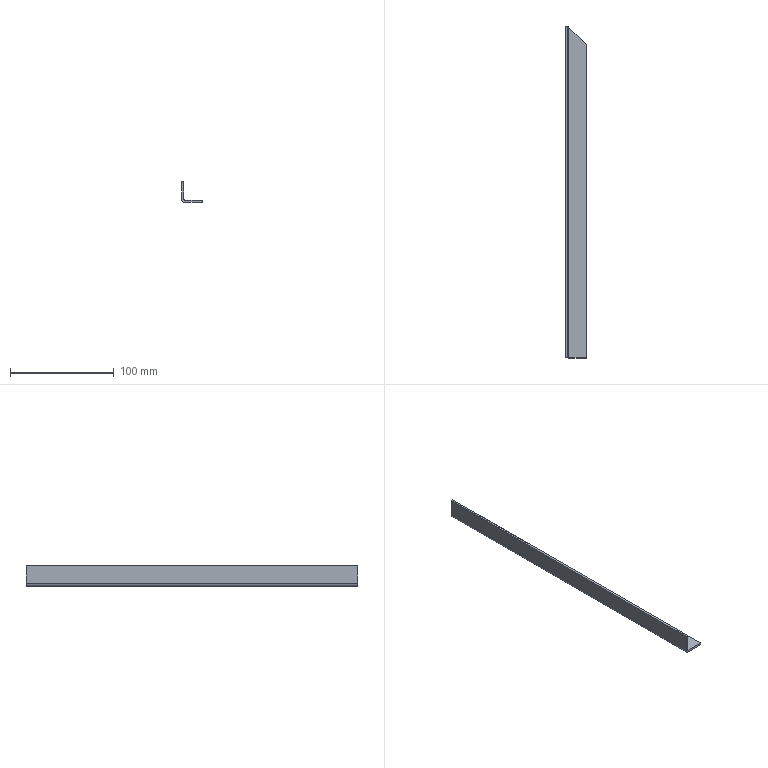Part | STEP file | Rear Closing Plate Frame Lower 3 | 1 solid | 12 faces | box 20 x 320 x 20 mm | volume 23444 mm3 | plane 9 | cylinder 2 | spline 1 | commonest cylinder face diameters 2 x1 6 x1
STEP:
#1=CARTESIAN_POINT('',(-1.251,25.392,3.));
#2=VERTEX_POINT('',#1);
#3=CARTESIAN_POINT('',(-1.251,25.392,20.));
#4=VERTEX_POINT('',#3);
#5=CARTESIAN_POINT('',(-1.251,25.392,0.));
#6=DIRECTION('',(0.,0.,1.));
#7=VECTOR('',#6,1000.);
#8=LINE('',#5,#7);
#9=EDGE_CURVE('',#2,#4,#8,.T.);
#10=ORIENTED_EDGE('',*,*,#9,.T.);
#11=CARTESIAN_POINT('',(-1.251,-294.608,20.));
#12=VERTEX_POINT('',#11);
#13=CARTESIAN_POINT('',(-1.251,0.,20.));
#14=DIRECTION('',(0.,-1.,0.));
#15=VECTOR('',#14,1000.);
#16=LINE('',#13,#15);
#17=EDGE_CURVE('',#4,#12,#16,.T.);
#18=ORIENTED_EDGE('',*,*,#17,.T.);
#19=CARTESIAN_POINT('',(-1.251,-294.608,3.));
#20=VERTEX_POINT('',#19);
#21=CARTESIAN_POINT('',(-1.251,-294.608,0.));
#22=DIRECTION('',(0.,0.,-1.));
#23=VECTOR('',#22,1000.);
#24=LINE('',#21,#23);
#25=EDGE_CURVE('',#12,#20,#24,.T.);
#26=ORIENTED_EDGE('',*,*,#25,.T.);
#27=CARTESIAN_POINT('',(-1.251,0.,3.));
#28=DIRECTION('',(0.,1.,0.));
#29=VECTOR('',#28,1000.);
#30=LINE('',#27,#29);
#31=EDGE_CURVE('',#20,#2,#30,.T.);
#32=ORIENTED_EDGE('',*,*,#31,.T.);
#33=EDGE_LOOP('',(#10,#18,#26,#32));
#34=FACE_OUTER_BOUND('',#33,.T.);
#35=CARTESIAN_POINT('',(-1.251,0.,0.));
#36=DIRECTION('',(1.,0.,0.));
#37=DIRECTION('',(0.,0.,-1.));
#38=AXIS2_PLACEMENT_3D('',#35,#36,#37);
#39=PLANE('',#38);
#40=ADVANCED_FACE('',(#34),#39,.T.);
#41=CARTESIAN_POINT('',(-3.251,25.392,20.));
#42=VERTEX_POINT('',#41);
#43=CARTESIAN_POINT('',(-3.251,25.392,20.));
#44=DIRECTION('',(1.,0.,0.));
#45=VECTOR('',#44,1000.);
#46=LINE('',#43,#45);
#47=EDGE_CURVE('',#42,#4,#46,.T.);
#48=ORIENTED_EDGE('',*,*,#47,.F.);
#49=CARTESIAN_POINT('',(-3.251,-294.608,20.));
#50=VERTEX_POINT('',#49);
#51=CARTESIAN_POINT('',(-3.251,25.392,20.));
#52=DIRECTION('',(0.,1.,0.));
#53=VECTOR('',#52,1000.);
#54=LINE('',#51,#53);
#55=EDGE_CURVE('',#50,#42,#54,.T.);
#56=ORIENTED_EDGE('',*,*,#55,.F.);
#57=CARTESIAN_POINT('',(-3.251,-294.608,20.));
#58=DIRECTION('',(-1.,0.,0.));
#59=VECTOR('',#58,1000.);
#60=LINE('',#57,#59);
#61=EDGE_CURVE('',#12,#50,#60,.T.);
#62=ORIENTED_EDGE('',*,*,#61,.F.);
#63=ORIENTED_EDGE('',*,*,#17,.F.);
#64=EDGE_LOOP('',(#48,#56,#62,#63));
#65=FACE_OUTER_BOUND('',#64,.T.);
#66=CARTESIAN_POINT('',(-3.251,25.392,20.));
#67=DIRECTION('',(0.,0.,-1.));
#68=DIRECTION('',(-1.,0.,0.));
#69=AXIS2_PLACEMENT_3D('',#66,#67,#68);
#70=PLANE('',#69);
#71=ADVANCED_FACE('',(#65),#70,.F.);
#72=CARTESIAN_POINT('',(-3.251,25.392,3.));
#73=VERTEX_POINT('',#72);
#74=CARTESIAN_POINT('',(-3.251,25.392,2.));
#75=DIRECTION('',(0.,0.,-1.));
#76=VECTOR('',#75,1000.);
#77=LINE('',#74,#76);
#78=EDGE_CURVE('',#42,#73,#77,.T.);
#79=ORIENTED_EDGE('',*,*,#78,.F.);
#80=ORIENTED_EDGE('',*,*,#47,.T.);
#81=ORIENTED_EDGE('',*,*,#9,.F.);
#82=CARTESIAN_POINT('',(-3.251,25.392,3.));
#83=DIRECTION('',(1.,0.,0.));
#84=VECTOR('',#83,1000.);
#85=LINE('',#82,#84);
#86=EDGE_CURVE('',#73,#2,#85,.T.);
#87=ORIENTED_EDGE('',*,*,#86,.F.);
#88=EDGE_LOOP('',(#79,#80,#81,#87));
#89=FACE_OUTER_BOUND('',#88,.T.);
#90=CARTESIAN_POINT('',(-3.251,25.392,2.));
#91=DIRECTION('',(0.,-1.,0.));
#92=DIRECTION('',(1.,0.,0.));
#93=AXIS2_PLACEMENT_3D('',#90,#91,#92);
#94=PLANE('',#93);
#95=ADVANCED_FACE('',(#89),#94,.F.);
#96=CARTESIAN_POINT('',(-0.2512,24.392,2.));
#97=VERTEX_POINT('',#96);
#98=CARTESIAN_POINT('',(-1.251,25.392,3.));
#99=CARTESIAN_POINT('',(-1.251,25.308,2.868));
#100=CARTESIAN_POINT('',(-1.226,25.226,2.74));
#101=CARTESIAN_POINT('',(-1.125,25.059,2.497));
#102=CARTESIAN_POINT('',(-1.052,24.976,2.387));
#103=CARTESIAN_POINT('',(-0.7735,24.725,2.108));
#104=CARTESIAN_POINT('',(-0.5154,24.56,2.));
#105=CARTESIAN_POINT('',(-0.2512,24.392,2.));
#106=B_SPLINE_CURVE_WITH_KNOTS('',3,(#98,#99,#100,#101,#102,#103,#104,#105),.UNSPECIFIED.,.F.,.F.,(4,2,2,4),(0.,0.0004622,0.0009244,0.001849),.UNSPECIFIED.);
#107=EDGE_CURVE('',#2,#97,#106,.T.);
#108=ORIENTED_EDGE('',*,*,#107,.F.);
#109=ORIENTED_EDGE('',*,*,#31,.F.);
#110=CARTESIAN_POINT('',(-0.2512,-294.608,2.));
#111=VERTEX_POINT('',#110);
#112=CARTESIAN_POINT('',(-0.2512,-294.608,3.));
#113=DIRECTION('',(0.,-1.,0.));
#114=DIRECTION('',(1.,0.,0.));
#115=AXIS2_PLACEMENT_3D('',#112,#113,#114);
#116=CIRCLE('',#115,1.);
#117=EDGE_CURVE('',#20,#111,#116,.T.);
#118=ORIENTED_EDGE('',*,*,#117,.T.);
#119=CARTESIAN_POINT('',(-0.2512,-294.608,2.));
#120=DIRECTION('',(0.,-1.,0.));
#121=VECTOR('',#120,1000.);
#122=LINE('',#119,#121);
#123=EDGE_CURVE('',#97,#111,#122,.T.);
#124=ORIENTED_EDGE('',*,*,#123,.F.);
#125=EDGE_LOOP('',(#108,#109,#118,#124));
#126=FACE_OUTER_BOUND('',#125,.T.);
#127=CARTESIAN_POINT('',(-0.2512,-294.608,3.));
#128=DIRECTION('',(0.,-1.,0.));
#129=DIRECTION('',(1.,0.,0.));
#130=AXIS2_PLACEMENT_3D('',#127,#128,#129);
#131=CYLINDRICAL_SURFACE('',#130,1.);
#132=ADVANCED_FACE('',(#126),#131,.F.);
#133=ORIENTED_EDGE('',*,*,#25,.F.);
#134=ORIENTED_EDGE('',*,*,#61,.T.);
#135=CARTESIAN_POINT('',(-3.251,-294.608,3.));
#136=VERTEX_POINT('',#135);
#137=CARTESIAN_POINT('',(-3.251,-294.608,20.));
#138=DIRECTION('',(0.,0.,1.));
#139=VECTOR('',#138,1000.);
#140=LINE('',#137,#139);
#141=EDGE_CURVE('',#136,#50,#140,.T.);
#142=ORIENTED_EDGE('',*,*,#141,.F.);
#143=CARTESIAN_POINT('',(-0.2512,-294.608,0.));
#144=VERTEX_POINT('',#143);
#145=CARTESIAN_POINT('',(-0.2512,-294.608,3.));
#146=DIRECTION('',(0.,1.,0.));
#147=DIRECTION('',(1.,0.,0.));
#148=AXIS2_PLACEMENT_3D('',#145,#146,#147);
#149=CIRCLE('',#148,3.);
#150=EDGE_CURVE('',#144,#136,#149,.T.);
#151=ORIENTED_EDGE('',*,*,#150,.F.);
#152=CARTESIAN_POINT('',(16.749,-294.608,0.));
#153=VERTEX_POINT('',#152);
#154=CARTESIAN_POINT('',(-3.251,-294.608,0.));
#155=DIRECTION('',(-1.,0.,0.));
#156=VECTOR('',#155,1000.);
#157=LINE('',#154,#156);
#158=EDGE_CURVE('',#153,#144,#157,.T.);
#159=ORIENTED_EDGE('',*,*,#158,.F.);
#160=CARTESIAN_POINT('',(16.749,-294.608,2.));
#161=VERTEX_POINT('',#160);
#162=CARTESIAN_POINT('',(16.749,-294.608,0.));
#163=DIRECTION('',(0.,0.,-1.));
#164=VECTOR('',#163,1000.);
#165=LINE('',#162,#164);
#166=EDGE_CURVE('',#161,#153,#165,.T.);
#167=ORIENTED_EDGE('',*,*,#166,.F.);
#168=CARTESIAN_POINT('',(0.,-294.608,2.));
#169=DIRECTION('',(-1.,0.,0.));
#170=VECTOR('',#169,1000.);
#171=LINE('',#168,#170);
#172=EDGE_CURVE('',#161,#111,#171,.T.);
#173=ORIENTED_EDGE('',*,*,#172,.T.);
#174=ORIENTED_EDGE('',*,*,#117,.F.);
#175=EDGE_LOOP('',(#133,#134,#142,#151,#159,#167,#173,#174));
#176=FACE_OUTER_BOUND('',#175,.T.);
#177=CARTESIAN_POINT('',(-3.251,-294.608,20.));
#178=DIRECTION('',(0.,1.,0.));
#179=DIRECTION('',(-1.,0.,0.));
#180=AXIS2_PLACEMENT_3D('',#177,#178,#179);
#181=PLANE('',#180);
#182=ADVANCED_FACE('',(#176),#181,.F.);
#183=ORIENTED_EDGE('',*,*,#141,.T.);
#184=ORIENTED_EDGE('',*,*,#55,.T.);
#185=ORIENTED_EDGE('',*,*,#78,.T.);
#186=CARTESIAN_POINT('',(-3.251,0.,3.));
#187=DIRECTION('',(0.,1.,0.));
#188=VECTOR('',#187,1000.);
#189=LINE('',#186,#188);
#190=EDGE_CURVE('',#136,#73,#189,.T.);
#191=ORIENTED_EDGE('',*,*,#190,.F.);
#192=EDGE_LOOP('',(#183,#184,#185,#191));
#193=FACE_OUTER_BOUND('',#192,.T.);
#194=CARTESIAN_POINT('',(-3.251,0.,0.));
#195=DIRECTION('',(1.,0.,0.));
#196=DIRECTION('',(0.,0.,-1.));
#197=AXIS2_PLACEMENT_3D('',#194,#195,#196);
#198=PLANE('',#197);
#199=ADVANCED_FACE('',(#193),#198,.F.);
#200=ORIENTED_EDGE('',*,*,#107,.T.);
#201=CARTESIAN_POINT('',(-0.2512,24.392,0.));
#202=VERTEX_POINT('',#201);
#203=CARTESIAN_POINT('',(-0.2512,24.392,1.));
#204=DIRECTION('',(0.,0.,1.));
#205=VECTOR('',#204,1000.);
#206=LINE('',#203,#205);
#207=EDGE_CURVE('',#202,#97,#206,.T.);
#208=ORIENTED_EDGE('',*,*,#207,.F.);
#209=CARTESIAN_POINT('',(-3.251,25.392,3.));
#210=CARTESIAN_POINT('',(-3.251,25.35,2.802));
#211=CARTESIAN_POINT('',(-3.232,25.308,2.607));
#212=CARTESIAN_POINT('',(-3.156,25.225,2.224));
#213=CARTESIAN_POINT('',(-3.098,25.183,2.034));
#214=CARTESIAN_POINT('',(-2.948,25.1,1.67));
#215=CARTESIAN_POINT('',(-2.855,25.059,1.498));
#216=CARTESIAN_POINT('',(-2.638,24.976,1.172));
#217=CARTESIAN_POINT('',(-2.512,24.933,1.018));
#218=CARTESIAN_POINT('',(-2.235,24.85,0.7409));
#219=CARTESIAN_POINT('',(-2.084,24.809,0.6168));
#220=CARTESIAN_POINT('',(-1.757,24.726,0.3979));
#221=CARTESIAN_POINT('',(-1.582,24.684,0.3042));
#222=CARTESIAN_POINT('',(-1.041,24.559,0.07951));
#223=CARTESIAN_POINT('',(-0.6473,24.476,0.));
#224=CARTESIAN_POINT('',(-0.2512,24.392,0.));
#225=B_SPLINE_CURVE_WITH_KNOTS('',3,(#209,#210,#211,#212,#213,#214,#215,#216,#217,#218,#219,#220,#221,#222,#223,#224),.UNSPECIFIED.,.F.,.F.,(4,2,2,2,2,2,2,4),(0.,0.000599,0.001198,0.001797,0.002396,0.002995,0.003594,0.004792),.UNSPECIFIED.);
#226=EDGE_CURVE('',#73,#202,#225,.T.);
#227=ORIENTED_EDGE('',*,*,#226,.F.);
#228=ORIENTED_EDGE('',*,*,#86,.T.);
#229=EDGE_LOOP('',(#200,#208,#227,#228));
#230=FACE_OUTER_BOUND('',#229,.T.);
#231=CARTESIAN_POINT('',(-0.2512,24.392,-0.02));
#232=CARTESIAN_POINT('',(-0.6466,24.475,-0.02));
#233=CARTESIAN_POINT('',(-1.042,24.558,0.0586));
#234=CARTESIAN_POINT('',(-1.772,24.725,0.3612));
#235=CARTESIAN_POINT('',(-2.107,24.808,0.585));
#236=CARTESIAN_POINT('',(-2.666,24.975,1.144));
#237=CARTESIAN_POINT('',(-2.89,25.058,1.479));
#238=CARTESIAN_POINT('',(-3.193,25.225,2.21));
#239=CARTESIAN_POINT('',(-3.271,25.308,2.605));
#240=CARTESIAN_POINT('',(-3.271,25.392,3.));
#241=CARTESIAN_POINT('',(-0.2512,24.392,0.));
#242=CARTESIAN_POINT('',(-0.6439,24.475,0.));
#243=CARTESIAN_POINT('',(-1.036,24.558,0.07808));
#244=CARTESIAN_POINT('',(-1.762,24.725,0.3786));
#245=CARTESIAN_POINT('',(-2.095,24.808,0.601));
#246=CARTESIAN_POINT('',(-2.65,24.975,1.156));
#247=CARTESIAN_POINT('',(-2.873,25.058,1.489));
#248=CARTESIAN_POINT('',(-3.173,25.225,2.215));
#249=CARTESIAN_POINT('',(-3.251,25.308,2.607));
#250=CARTESIAN_POINT('',(-3.251,25.392,3.));
#251=CARTESIAN_POINT('',(-0.2512,24.392,2.));
#252=CARTESIAN_POINT('',(-0.3821,24.475,2.));
#253=CARTESIAN_POINT('',(-0.5129,24.558,2.026));
#254=CARTESIAN_POINT('',(-0.7548,24.725,2.126));
#255=CARTESIAN_POINT('',(-0.8657,24.808,2.2));
#256=CARTESIAN_POINT('',(-1.051,24.975,2.385));
#257=CARTESIAN_POINT('',(-1.125,25.058,2.496));
#258=CARTESIAN_POINT('',(-1.225,25.225,2.738));
#259=CARTESIAN_POINT('',(-1.251,25.308,2.869));
#260=CARTESIAN_POINT('',(-1.251,25.392,3.));
#261=CARTESIAN_POINT('',(-0.2512,24.392,2.02));
#262=CARTESIAN_POINT('',(-0.3794,24.475,2.02));
#263=CARTESIAN_POINT('',(-0.5076,24.558,2.046));
#264=CARTESIAN_POINT('',(-0.7446,24.725,2.144));
#265=CARTESIAN_POINT('',(-0.8533,24.808,2.216));
#266=CARTESIAN_POINT('',(-1.035,24.975,2.398));
#267=CARTESIAN_POINT('',(-1.107,25.058,2.507));
#268=CARTESIAN_POINT('',(-1.205,25.225,2.744));
#269=CARTESIAN_POINT('',(-1.231,25.308,2.872));
#270=CARTESIAN_POINT('',(-1.231,25.392,3.));
#271=B_SPLINE_SURFACE_WITH_KNOTS('',1,3,((#231,#232,#233,#234,#235,#236,#237,#238,#239,#240),(#241,#242,#243,#244,#245,#246,#247,#248,#249,#250),(#251,#252,#253,#254,#255,#256,#257,#258,#259,#260),(#261,#262,#263,#264,#265,#266,#267,#268,#269,#270)),.UNSPECIFIED.,.F.,.F.,.F.,(2,1,1,2),(4,2,2,2,4),(-0.01,0.,1.,1.01),(0.,0.25,0.5,0.75,1.),.UNSPECIFIED.);
#272=ADVANCED_FACE('',(#230),#271,.F.);
#273=ORIENTED_EDGE('',*,*,#172,.F.);
#274=CARTESIAN_POINT('',(16.749,7.392,2.));
#275=VERTEX_POINT('',#274);
#276=CARTESIAN_POINT('',(16.749,0.,2.));
#277=DIRECTION('',(0.,-1.,0.));
#278=VECTOR('',#277,1000.);
#279=LINE('',#276,#278);
#280=EDGE_CURVE('',#275,#161,#279,.T.);
#281=ORIENTED_EDGE('',*,*,#280,.F.);
#282=CARTESIAN_POINT('',(-0.2512,24.392,2.));
#283=DIRECTION('',(0.7071,-0.7071,0.));
#284=VECTOR('',#283,1000.);
#285=LINE('',#282,#284);
#286=EDGE_CURVE('',#97,#275,#285,.T.);
#287=ORIENTED_EDGE('',*,*,#286,.F.);
#288=ORIENTED_EDGE('',*,*,#123,.T.);
#289=EDGE_LOOP('',(#273,#281,#287,#288));
#290=FACE_OUTER_BOUND('',#289,.T.);
#291=CARTESIAN_POINT('',(0.,0.,2.));
#292=DIRECTION('',(0.,0.,-1.));
#293=DIRECTION('',(-1.,0.,0.));
#294=AXIS2_PLACEMENT_3D('',#291,#292,#293);
#295=PLANE('',#294);
#296=ADVANCED_FACE('',(#290),#295,.F.);
#297=ORIENTED_EDGE('',*,*,#190,.T.);
#298=ORIENTED_EDGE('',*,*,#226,.T.);
#299=CARTESIAN_POINT('',(-0.2512,-294.608,0.));
#300=DIRECTION('',(0.,-1.,0.));
#301=VECTOR('',#300,1000.);
#302=LINE('',#299,#301);
#303=EDGE_CURVE('',#202,#144,#302,.T.);
#304=ORIENTED_EDGE('',*,*,#303,.T.);
#305=ORIENTED_EDGE('',*,*,#150,.T.);
#306=EDGE_LOOP('',(#297,#298,#304,#305));
#307=FACE_OUTER_BOUND('',#306,.T.);
#308=CARTESIAN_POINT('',(-0.2512,-294.608,3.));
#309=DIRECTION('',(0.,-1.,0.));
#310=DIRECTION('',(1.,0.,0.));
#311=AXIS2_PLACEMENT_3D('',#308,#309,#310);
#312=CYLINDRICAL_SURFACE('',#311,3.);
#313=ADVANCED_FACE('',(#307),#312,.T.);
#314=ORIENTED_EDGE('',*,*,#207,.T.);
#315=ORIENTED_EDGE('',*,*,#286,.T.);
#316=CARTESIAN_POINT('',(16.749,7.392,0.));
#317=VERTEX_POINT('',#316);
#318=CARTESIAN_POINT('',(16.749,7.392,0.));
#319=DIRECTION('',(0.,0.,1.));
#320=VECTOR('',#319,1000.);
#321=LINE('',#318,#320);
#322=EDGE_CURVE('',#317,#275,#321,.T.);
#323=ORIENTED_EDGE('',*,*,#322,.F.);
#324=CARTESIAN_POINT('',(-1.251,25.392,0.));
#325=DIRECTION('',(0.7071,-0.7071,0.));
#326=VECTOR('',#325,1000.);
#327=LINE('',#324,#326);
#328=EDGE_CURVE('',#202,#317,#327,.T.);
#329=ORIENTED_EDGE('',*,*,#328,.F.);
#330=EDGE_LOOP('',(#314,#315,#323,#329));
#331=FACE_OUTER_BOUND('',#330,.T.);
#332=CARTESIAN_POINT('',(-1.251,25.392,0.));
#333=DIRECTION('',(-0.7071,-0.7071,0.));
#334=DIRECTION('',(0.7071,-0.7071,0.));
#335=AXIS2_PLACEMENT_3D('',#332,#333,#334);
#336=PLANE('',#335);
#337=ADVANCED_FACE('',(#331),#336,.F.);
#338=ORIENTED_EDGE('',*,*,#166,.T.);
#339=CARTESIAN_POINT('',(16.749,7.392,0.));
#340=DIRECTION('',(0.,1.,0.));
#341=VECTOR('',#340,1000.);
#342=LINE('',#339,#341);
#343=EDGE_CURVE('',#153,#317,#342,.T.);
#344=ORIENTED_EDGE('',*,*,#343,.T.);
#345=ORIENTED_EDGE('',*,*,#322,.T.);
#346=ORIENTED_EDGE('',*,*,#280,.T.);
#347=EDGE_LOOP('',(#338,#344,#345,#346));
#348=FACE_OUTER_BOUND('',#347,.T.);
#349=CARTESIAN_POINT('',(16.749,7.392,0.));
#350=DIRECTION('',(1.,0.,0.));
#351=DIRECTION('',(0.,1.,0.));
#352=AXIS2_PLACEMENT_3D('',#349,#350,#351);
#353=PLANE('',#352);
#354=ADVANCED_FACE('',(#348),#353,.T.);
#355=ORIENTED_EDGE('',*,*,#328,.T.);
#356=ORIENTED_EDGE('',*,*,#343,.F.);
#357=ORIENTED_EDGE('',*,*,#158,.T.);
#358=ORIENTED_EDGE('',*,*,#303,.F.);
#359=EDGE_LOOP('',(#355,#356,#357,#358));
#360=FACE_OUTER_BOUND('',#359,.T.);
#361=CARTESIAN_POINT('',(0.,0.,0.));
#362=DIRECTION('',(0.,0.,-1.));
#363=DIRECTION('',(-1.,0.,0.));
#364=AXIS2_PLACEMENT_3D('',#361,#362,#363);
#365=PLANE('',#364);
#366=ADVANCED_FACE('',(#360),#365,.T.);
#367=CLOSED_SHELL('',(#40,#71,#95,#132,#182,#199,#272,#296,#313,#337,#354,#366));
#368=MANIFOLD_SOLID_BREP('',#367);
#369=CARTESIAN_POINT('',(0.,0.,0.));
#370=DIRECTION('',(0.,0.,1.));
#371=DIRECTION('',(1.,0.,0.));
#372=AXIS2_PLACEMENT_3D('',#369,#370,#371);
#373=(LENGTH_UNIT()NAMED_UNIT(*)SI_UNIT(.MILLI.,.METRE.));
#374=UNCERTAINTY_MEASURE_WITH_UNIT(LENGTH_MEASURE(0.00001),#373,'','');
#375=(NAMED_UNIT(*)PLANE_ANGLE_UNIT()SI_UNIT($,.RADIAN.));
#376=(NAMED_UNIT(*)SI_UNIT($,.STERADIAN.)SOLID_ANGLE_UNIT());
#377=(GEOMETRIC_REPRESENTATION_CONTEXT(3)GLOBAL_UNCERTAINTY_ASSIGNED_CONTEXT((#374))GLOBAL_UNIT_ASSIGNED_CONTEXT((#373,#375,#376))REPRESENTATION_CONTEXT('',''));
#378=ADVANCED_BREP_SHAPE_REPRESENTATION('',(#368,#372),#377);